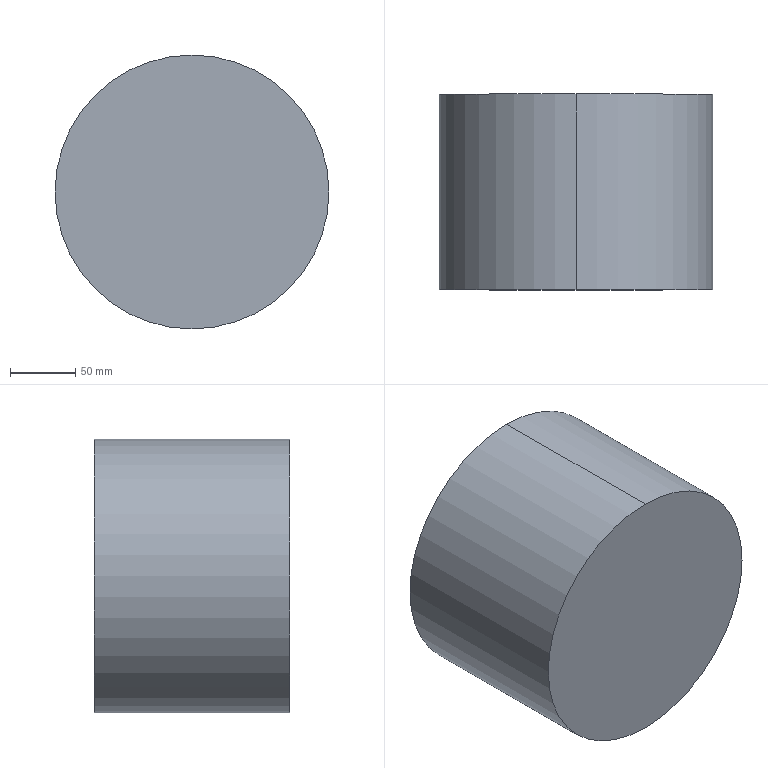Part | STEP file | X77-01302 | 1 solid | 8 faces | box 210 x 150 x 210 mm | volume 329352 mm3 | cylinder 4 | plane 4 | commonest cylinder face diameters 206 x2 210 x2
STEP:
#1=CARTESIAN_POINT('',(0.,150.,105.));
#2=VERTEX_POINT('',#1);
#3=CARTESIAN_POINT('',(0.,150.,-105.));
#4=VERTEX_POINT('',#3);
#5=CARTESIAN_POINT('',(0.,150.,0.));
#6=DIRECTION('',(0.,1.,0.));
#7=DIRECTION('',(0.,0.,1.));
#8=AXIS2_PLACEMENT_3D('',#5,#6,#7);
#9=CIRCLE('',#8,105.);
#10=EDGE_CURVE('',#2,#4,#9,.T.);
#11=ORIENTED_EDGE('',*,*,#10,.F.);
#12=CARTESIAN_POINT('',(0.,0.,105.));
#13=VERTEX_POINT('',#12);
#14=CARTESIAN_POINT('',(0.,150.,105.));
#15=DIRECTION('',(0.,-1.,0.));
#16=VECTOR('',#15,1000.);
#17=LINE('',#14,#16);
#18=EDGE_CURVE('',#2,#13,#17,.T.);
#19=ORIENTED_EDGE('',*,*,#18,.T.);
#20=CARTESIAN_POINT('',(0.,0.,-105.));
#21=VERTEX_POINT('',#20);
#22=CARTESIAN_POINT('',(0.,0.,0.));
#23=DIRECTION('',(0.,1.,0.));
#24=DIRECTION('',(0.,0.,1.));
#25=AXIS2_PLACEMENT_3D('',#22,#23,#24);
#26=CIRCLE('',#25,105.);
#27=EDGE_CURVE('',#13,#21,#26,.T.);
#28=ORIENTED_EDGE('',*,*,#27,.T.);
#29=CARTESIAN_POINT('',(0.,150.,-105.));
#30=DIRECTION('',(0.,-1.,0.));
#31=VECTOR('',#30,1000.);
#32=LINE('',#29,#31);
#33=EDGE_CURVE('',#4,#21,#32,.T.);
#34=ORIENTED_EDGE('',*,*,#33,.F.);
#35=EDGE_LOOP('',(#11,#19,#28,#34));
#36=FACE_OUTER_BOUND('',#35,.T.);
#37=CARTESIAN_POINT('',(0.,150.,0.));
#38=DIRECTION('',(0.,-1.,0.));
#39=DIRECTION('',(0.,0.,-1.));
#40=AXIS2_PLACEMENT_3D('',#37,#38,#39);
#41=CYLINDRICAL_SURFACE('',#40,105.);
#42=ADVANCED_FACE('',(#36),#41,.T.);
#43=ORIENTED_EDGE('',*,*,#18,.F.);
#44=CARTESIAN_POINT('',(0.,150.,0.));
#45=DIRECTION('',(0.,1.,0.));
#46=DIRECTION('',(0.,0.,1.));
#47=AXIS2_PLACEMENT_3D('',#44,#45,#46);
#48=CIRCLE('',#47,105.);
#49=EDGE_CURVE('',#4,#2,#48,.T.);
#50=ORIENTED_EDGE('',*,*,#49,.F.);
#51=ORIENTED_EDGE('',*,*,#33,.T.);
#52=CARTESIAN_POINT('',(0.,0.,0.));
#53=DIRECTION('',(0.,1.,0.));
#54=DIRECTION('',(0.,0.,1.));
#55=AXIS2_PLACEMENT_3D('',#52,#53,#54);
#56=CIRCLE('',#55,105.);
#57=EDGE_CURVE('',#21,#13,#56,.T.);
#58=ORIENTED_EDGE('',*,*,#57,.T.);
#59=EDGE_LOOP('',(#43,#50,#51,#58));
#60=FACE_OUTER_BOUND('',#59,.T.);
#61=CARTESIAN_POINT('',(0.,150.,0.));
#62=DIRECTION('',(0.,-1.,0.));
#63=DIRECTION('',(0.,0.,-1.));
#64=AXIS2_PLACEMENT_3D('',#61,#62,#63);
#65=CYLINDRICAL_SURFACE('',#64,105.);
#66=ADVANCED_FACE('',(#60),#65,.T.);
#67=ORIENTED_EDGE('',*,*,#49,.T.);
#68=ORIENTED_EDGE('',*,*,#10,.T.);
#69=EDGE_LOOP('',(#67,#68));
#70=FACE_OUTER_BOUND('',#69,.T.);
#71=CARTESIAN_POINT('',(0.,150.,0.));
#72=DIRECTION('',(0.,1.,0.));
#73=DIRECTION('',(0.,0.,1.));
#74=AXIS2_PLACEMENT_3D('',#71,#72,#73);
#75=PLANE('',#74);
#76=ADVANCED_FACE('',(#70),#75,.T.);
#77=ORIENTED_EDGE('',*,*,#57,.F.);
#78=ORIENTED_EDGE('',*,*,#27,.F.);
#79=EDGE_LOOP('',(#77,#78));
#80=FACE_OUTER_BOUND('',#79,.T.);
#81=CARTESIAN_POINT('',(0.,0.,0.));
#82=DIRECTION('',(0.,1.,0.));
#83=DIRECTION('',(0.,0.,1.));
#84=AXIS2_PLACEMENT_3D('',#81,#82,#83);
#85=PLANE('',#84);
#86=ADVANCED_FACE('',(#80),#85,.F.);
#87=CLOSED_SHELL('',(#42,#66,#76,#86));
#88=CARTESIAN_POINT('',(0.,148.,-103.));
#89=VERTEX_POINT('',#88);
#90=CARTESIAN_POINT('',(0.,148.,103.));
#91=VERTEX_POINT('',#90);
#92=CARTESIAN_POINT('',(0.,148.,0.));
#93=DIRECTION('',(0.,1.,0.));
#94=DIRECTION('',(0.,0.,1.));
#95=AXIS2_PLACEMENT_3D('',#92,#93,#94);
#96=CIRCLE('',#95,103.);
#97=EDGE_CURVE('',#89,#91,#96,.T.);
#98=ORIENTED_EDGE('',*,*,#97,.T.);
#99=CARTESIAN_POINT('',(0.,2.,103.));
#100=VERTEX_POINT('',#99);
#101=CARTESIAN_POINT('',(0.,150.,103.));
#102=DIRECTION('',(0.,-1.,0.));
#103=VECTOR('',#102,1000.);
#104=LINE('',#101,#103);
#105=EDGE_CURVE('',#91,#100,#104,.T.);
#106=ORIENTED_EDGE('',*,*,#105,.T.);
#107=CARTESIAN_POINT('',(0.,2.,-103.));
#108=VERTEX_POINT('',#107);
#109=CARTESIAN_POINT('',(0.,2.,0.));
#110=DIRECTION('',(0.,1.,0.));
#111=DIRECTION('',(0.,0.,1.));
#112=AXIS2_PLACEMENT_3D('',#109,#110,#111);
#113=CIRCLE('',#112,103.);
#114=EDGE_CURVE('',#108,#100,#113,.T.);
#115=ORIENTED_EDGE('',*,*,#114,.F.);
#116=CARTESIAN_POINT('',(0.,150.,-103.));
#117=DIRECTION('',(0.,-1.,0.));
#118=VECTOR('',#117,1000.);
#119=LINE('',#116,#118);
#120=EDGE_CURVE('',#89,#108,#119,.T.);
#121=ORIENTED_EDGE('',*,*,#120,.F.);
#122=EDGE_LOOP('',(#98,#106,#115,#121));
#123=FACE_OUTER_BOUND('',#122,.T.);
#124=CARTESIAN_POINT('',(0.,150.,0.));
#125=DIRECTION('',(0.,-1.,0.));
#126=DIRECTION('',(0.,0.,-1.));
#127=AXIS2_PLACEMENT_3D('',#124,#125,#126);
#128=CYLINDRICAL_SURFACE('',#127,103.);
#129=ADVANCED_FACE('',(#123),#128,.F.);
#130=ORIENTED_EDGE('',*,*,#97,.F.);
#131=CARTESIAN_POINT('',(0.,148.,0.));
#132=DIRECTION('',(0.,1.,0.));
#133=DIRECTION('',(0.,0.,1.));
#134=AXIS2_PLACEMENT_3D('',#131,#132,#133);
#135=CIRCLE('',#134,103.);
#136=EDGE_CURVE('',#91,#89,#135,.T.);
#137=ORIENTED_EDGE('',*,*,#136,.F.);
#138=EDGE_LOOP('',(#130,#137));
#139=FACE_OUTER_BOUND('',#138,.T.);
#140=CARTESIAN_POINT('',(0.,148.,0.));
#141=DIRECTION('',(0.,1.,0.));
#142=DIRECTION('',(0.,0.,1.));
#143=AXIS2_PLACEMENT_3D('',#140,#141,#142);
#144=PLANE('',#143);
#145=ADVANCED_FACE('',(#139),#144,.F.);
#146=ORIENTED_EDGE('',*,*,#114,.T.);
#147=CARTESIAN_POINT('',(0.,2.,0.));
#148=DIRECTION('',(0.,1.,0.));
#149=DIRECTION('',(0.,0.,1.));
#150=AXIS2_PLACEMENT_3D('',#147,#148,#149);
#151=CIRCLE('',#150,103.);
#152=EDGE_CURVE('',#100,#108,#151,.T.);
#153=ORIENTED_EDGE('',*,*,#152,.T.);
#154=EDGE_LOOP('',(#146,#153));
#155=FACE_OUTER_BOUND('',#154,.T.);
#156=CARTESIAN_POINT('',(0.,2.,0.));
#157=DIRECTION('',(0.,1.,0.));
#158=DIRECTION('',(0.,0.,1.));
#159=AXIS2_PLACEMENT_3D('',#156,#157,#158);
#160=PLANE('',#159);
#161=ADVANCED_FACE('',(#155),#160,.T.);
#162=ORIENTED_EDGE('',*,*,#105,.F.);
#163=ORIENTED_EDGE('',*,*,#136,.T.);
#164=ORIENTED_EDGE('',*,*,#120,.T.);
#165=ORIENTED_EDGE('',*,*,#152,.F.);
#166=EDGE_LOOP('',(#162,#163,#164,#165));
#167=FACE_OUTER_BOUND('',#166,.T.);
#168=CARTESIAN_POINT('',(0.,150.,0.));
#169=DIRECTION('',(0.,-1.,0.));
#170=DIRECTION('',(0.,0.,-1.));
#171=AXIS2_PLACEMENT_3D('',#168,#169,#170);
#172=CYLINDRICAL_SURFACE('',#171,103.);
#173=ADVANCED_FACE('',(#167),#172,.F.);
#174=CLOSED_SHELL('',(#129,#145,#161,#173));
#175=ORIENTED_CLOSED_SHELL('',*,#174,.F.);
#176=BREP_WITH_VOIDS('',#87,(#175));
#177=CARTESIAN_POINT('',(0.,0.,0.));
#178=DIRECTION('',(0.,0.,1.));
#179=DIRECTION('',(1.,0.,0.));
#180=AXIS2_PLACEMENT_3D('',#177,#178,#179);
#181=(LENGTH_UNIT()NAMED_UNIT(*)SI_UNIT(.MILLI.,.METRE.));
#182=UNCERTAINTY_MEASURE_WITH_UNIT(LENGTH_MEASURE(0.00001),#181,'','');
#183=(NAMED_UNIT(*)PLANE_ANGLE_UNIT()SI_UNIT($,.RADIAN.));
#184=(NAMED_UNIT(*)SI_UNIT($,.STERADIAN.)SOLID_ANGLE_UNIT());
#185=(GEOMETRIC_REPRESENTATION_CONTEXT(3)GLOBAL_UNCERTAINTY_ASSIGNED_CONTEXT((#182))GLOBAL_UNIT_ASSIGNED_CONTEXT((#181,#183,#184))REPRESENTATION_CONTEXT('',''));
#186=ADVANCED_BREP_SHAPE_REPRESENTATION('',(#176,#180),#185);